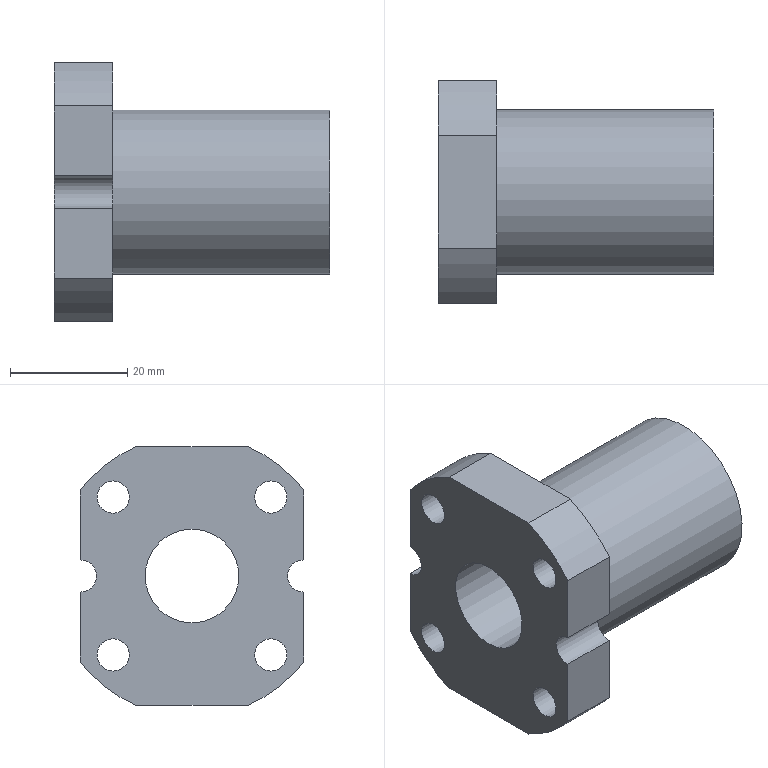Part | NX | 1 solid | 21 faces | box 47 x 38 x 44 mm | volume 27725 mm3 | cylinder 12 | plane 9 | commonest cylinder face diameters 5.5 x6 48 x4 16 x1 28 x1
STEP:
#1=CARTESIAN_POINT('',(0.,19.,14.663));
#2=VERTEX_POINT('',#1);
#3=CARTESIAN_POINT('',(0.,19.,2.75));
#4=VERTEX_POINT('',#3);
#5=CARTESIAN_POINT('',(0.,19.,14.663));
#6=DIRECTION('',(0.,0.,-1.));
#7=VECTOR('',#6,1.);
#8=LINE('',#5,#7);
#9=EDGE_CURVE('',#2,#4,#8,.T.);
#10=ORIENTED_EDGE('',*,*,#9,.F.);
#11=CARTESIAN_POINT('',(10.,19.,14.663));
#12=VERTEX_POINT('',#11);
#13=CARTESIAN_POINT('',(10.,19.,14.663));
#14=DIRECTION('',(-1.,0.,0.));
#15=VECTOR('',#14,1.);
#16=LINE('',#13,#15);
#17=EDGE_CURVE('',#12,#2,#16,.T.);
#18=ORIENTED_EDGE('',*,*,#17,.F.);
#19=CARTESIAN_POINT('',(10.,19.,2.75));
#20=VERTEX_POINT('',#19);
#21=CARTESIAN_POINT('',(10.,19.,14.663));
#22=DIRECTION('',(0.,0.,-1.));
#23=VECTOR('',#22,1.);
#24=LINE('',#21,#23);
#25=EDGE_CURVE('',#12,#20,#24,.T.);
#26=ORIENTED_EDGE('',*,*,#25,.T.);
#27=CARTESIAN_POINT('',(10.,19.,2.75));
#28=DIRECTION('',(-1.,0.,0.));
#29=VECTOR('',#28,1.);
#30=LINE('',#27,#29);
#31=EDGE_CURVE('',#20,#4,#30,.T.);
#32=ORIENTED_EDGE('',*,*,#31,.T.);
#33=EDGE_LOOP('',(#10,#18,#26,#32));
#34=FACE_OUTER_BOUND('',#33,.T.);
#35=CARTESIAN_POINT('',(10.,19.,14.663));
#36=DIRECTION('',(0.,1.,0.));
#37=DIRECTION('',(0.,0.,-1.));
#38=AXIS2_PLACEMENT_3D('',#35,#36,#37);
#39=PLANE('',#38);
#40=ADVANCED_FACE('',(#34),#39,.T.);
#41=CARTESIAN_POINT('',(0.,19.,-2.75));
#42=VERTEX_POINT('',#41);
#43=CARTESIAN_POINT('',(0.,19.,0.));
#44=DIRECTION('',(1.,0.,0.));
#45=DIRECTION('',(0.,0.,-1.));
#46=AXIS2_PLACEMENT_3D('',#43,#44,#45);
#47=CIRCLE('',#46,2.75);
#48=EDGE_CURVE('',#4,#42,#47,.T.);
#49=ORIENTED_EDGE('',*,*,#48,.F.);
#50=ORIENTED_EDGE('',*,*,#31,.F.);
#51=CARTESIAN_POINT('',(10.,19.,-2.75));
#52=VERTEX_POINT('',#51);
#53=CARTESIAN_POINT('',(10.,19.,0.));
#54=DIRECTION('',(1.,0.,0.));
#55=DIRECTION('',(0.,0.,-1.));
#56=AXIS2_PLACEMENT_3D('',#53,#54,#55);
#57=CIRCLE('',#56,2.75);
#58=EDGE_CURVE('',#20,#52,#57,.T.);
#59=ORIENTED_EDGE('',*,*,#58,.T.);
#60=CARTESIAN_POINT('',(10.,19.,-2.75));
#61=DIRECTION('',(-1.,0.,0.));
#62=VECTOR('',#61,1.);
#63=LINE('',#60,#62);
#64=EDGE_CURVE('',#52,#42,#63,.T.);
#65=ORIENTED_EDGE('',*,*,#64,.T.);
#66=EDGE_LOOP('',(#49,#50,#59,#65));
#67=FACE_OUTER_BOUND('',#66,.T.);
#68=CARTESIAN_POINT('',(10.,19.,0.));
#69=DIRECTION('',(-1.,0.,0.));
#70=DIRECTION('',(0.,0.,-1.));
#71=AXIS2_PLACEMENT_3D('',#68,#69,#70);
#72=CYLINDRICAL_SURFACE('',#71,2.75);
#73=ADVANCED_FACE('',(#67),#72,.F.);
#74=CARTESIAN_POINT('',(0.,19.,-14.663));
#75=VERTEX_POINT('',#74);
#76=CARTESIAN_POINT('',(0.,19.,-2.75));
#77=DIRECTION('',(0.,0.,-1.));
#78=VECTOR('',#77,1.);
#79=LINE('',#76,#78);
#80=EDGE_CURVE('',#42,#75,#79,.T.);
#81=ORIENTED_EDGE('',*,*,#80,.F.);
#82=ORIENTED_EDGE('',*,*,#64,.F.);
#83=CARTESIAN_POINT('',(10.,19.,-14.663));
#84=VERTEX_POINT('',#83);
#85=CARTESIAN_POINT('',(10.,19.,-2.75));
#86=DIRECTION('',(0.,0.,-1.));
#87=VECTOR('',#86,1.);
#88=LINE('',#85,#87);
#89=EDGE_CURVE('',#52,#84,#88,.T.);
#90=ORIENTED_EDGE('',*,*,#89,.T.);
#91=CARTESIAN_POINT('',(10.,19.,-14.663));
#92=DIRECTION('',(-1.,0.,0.));
#93=VECTOR('',#92,1.);
#94=LINE('',#91,#93);
#95=EDGE_CURVE('',#84,#75,#94,.T.);
#96=ORIENTED_EDGE('',*,*,#95,.T.);
#97=EDGE_LOOP('',(#81,#82,#90,#96));
#98=FACE_OUTER_BOUND('',#97,.T.);
#99=CARTESIAN_POINT('',(10.,19.,-2.75));
#100=DIRECTION('',(0.,1.,0.));
#101=DIRECTION('',(0.,0.,-1.));
#102=AXIS2_PLACEMENT_3D('',#99,#100,#101);
#103=PLANE('',#102);
#104=ADVANCED_FACE('',(#98),#103,.T.);
#105=CARTESIAN_POINT('',(0.,9.592,-22.));
#106=VERTEX_POINT('',#105);
#107=CARTESIAN_POINT('',(0.,0.,0.));
#108=DIRECTION('',(-1.,0.,0.));
#109=DIRECTION('',(0.,0.,-1.));
#110=AXIS2_PLACEMENT_3D('',#107,#108,#109);
#111=CIRCLE('',#110,24.);
#112=EDGE_CURVE('',#75,#106,#111,.T.);
#113=ORIENTED_EDGE('',*,*,#112,.F.);
#114=ORIENTED_EDGE('',*,*,#95,.F.);
#115=CARTESIAN_POINT('',(10.,9.592,-22.));
#116=VERTEX_POINT('',#115);
#117=CARTESIAN_POINT('',(10.,0.,0.));
#118=DIRECTION('',(-1.,0.,0.));
#119=DIRECTION('',(0.,0.,-1.));
#120=AXIS2_PLACEMENT_3D('',#117,#118,#119);
#121=CIRCLE('',#120,24.);
#122=EDGE_CURVE('',#84,#116,#121,.T.);
#123=ORIENTED_EDGE('',*,*,#122,.T.);
#124=CARTESIAN_POINT('',(10.,9.592,-22.));
#125=DIRECTION('',(-1.,0.,0.));
#126=VECTOR('',#125,1.);
#127=LINE('',#124,#126);
#128=EDGE_CURVE('',#116,#106,#127,.T.);
#129=ORIENTED_EDGE('',*,*,#128,.T.);
#130=EDGE_LOOP('',(#113,#114,#123,#129));
#131=FACE_OUTER_BOUND('',#130,.T.);
#132=CARTESIAN_POINT('',(10.,0.,0.));
#133=DIRECTION('',(-1.,0.,0.));
#134=DIRECTION('',(0.,0.,-1.));
#135=AXIS2_PLACEMENT_3D('',#132,#133,#134);
#136=CYLINDRICAL_SURFACE('',#135,24.);
#137=ADVANCED_FACE('',(#131),#136,.T.);
#138=CARTESIAN_POINT('',(0.,-9.592,-22.));
#139=VERTEX_POINT('',#138);
#140=CARTESIAN_POINT('',(0.,9.592,-22.));
#141=DIRECTION('',(0.,-1.,0.));
#142=VECTOR('',#141,1.);
#143=LINE('',#140,#142);
#144=EDGE_CURVE('',#106,#139,#143,.T.);
#145=ORIENTED_EDGE('',*,*,#144,.F.);
#146=ORIENTED_EDGE('',*,*,#128,.F.);
#147=CARTESIAN_POINT('',(10.,-9.592,-22.));
#148=VERTEX_POINT('',#147);
#149=CARTESIAN_POINT('',(10.,9.592,-22.));
#150=DIRECTION('',(0.,-1.,0.));
#151=VECTOR('',#150,1.);
#152=LINE('',#149,#151);
#153=EDGE_CURVE('',#116,#148,#152,.T.);
#154=ORIENTED_EDGE('',*,*,#153,.T.);
#155=CARTESIAN_POINT('',(10.,-9.592,-22.));
#156=DIRECTION('',(-1.,0.,0.));
#157=VECTOR('',#156,1.);
#158=LINE('',#155,#157);
#159=EDGE_CURVE('',#148,#139,#158,.T.);
#160=ORIENTED_EDGE('',*,*,#159,.T.);
#161=EDGE_LOOP('',(#145,#146,#154,#160));
#162=FACE_OUTER_BOUND('',#161,.T.);
#163=CARTESIAN_POINT('',(10.,9.592,-22.));
#164=DIRECTION('',(0.,0.,-1.));
#165=DIRECTION('',(0.,-1.,0.));
#166=AXIS2_PLACEMENT_3D('',#163,#164,#165);
#167=PLANE('',#166);
#168=ADVANCED_FACE('',(#162),#167,.T.);
#169=CARTESIAN_POINT('',(0.,-19.,-14.663));
#170=VERTEX_POINT('',#169);
#171=CARTESIAN_POINT('',(0.,0.,0.));
#172=DIRECTION('',(-1.,0.,0.));
#173=DIRECTION('',(0.,0.,-1.));
#174=AXIS2_PLACEMENT_3D('',#171,#172,#173);
#175=CIRCLE('',#174,24.);
#176=EDGE_CURVE('',#139,#170,#175,.T.);
#177=ORIENTED_EDGE('',*,*,#176,.F.);
#178=ORIENTED_EDGE('',*,*,#159,.F.);
#179=CARTESIAN_POINT('',(10.,-19.,-14.663));
#180=VERTEX_POINT('',#179);
#181=CARTESIAN_POINT('',(10.,0.,0.));
#182=DIRECTION('',(-1.,0.,0.));
#183=DIRECTION('',(0.,0.,-1.));
#184=AXIS2_PLACEMENT_3D('',#181,#182,#183);
#185=CIRCLE('',#184,24.);
#186=EDGE_CURVE('',#148,#180,#185,.T.);
#187=ORIENTED_EDGE('',*,*,#186,.T.);
#188=CARTESIAN_POINT('',(10.,-19.,-14.663));
#189=DIRECTION('',(-1.,0.,0.));
#190=VECTOR('',#189,1.);
#191=LINE('',#188,#190);
#192=EDGE_CURVE('',#180,#170,#191,.T.);
#193=ORIENTED_EDGE('',*,*,#192,.T.);
#194=EDGE_LOOP('',(#177,#178,#187,#193));
#195=FACE_OUTER_BOUND('',#194,.T.);
#196=CARTESIAN_POINT('',(10.,0.,0.));
#197=DIRECTION('',(-1.,0.,0.));
#198=DIRECTION('',(0.,0.,-1.));
#199=AXIS2_PLACEMENT_3D('',#196,#197,#198);
#200=CYLINDRICAL_SURFACE('',#199,24.);
#201=ADVANCED_FACE('',(#195),#200,.T.);
#202=CARTESIAN_POINT('',(0.,-19.,-2.75));
#203=VERTEX_POINT('',#202);
#204=CARTESIAN_POINT('',(0.,-19.,-14.663));
#205=DIRECTION('',(0.,0.,1.));
#206=VECTOR('',#205,1.);
#207=LINE('',#204,#206);
#208=EDGE_CURVE('',#170,#203,#207,.T.);
#209=ORIENTED_EDGE('',*,*,#208,.F.);
#210=ORIENTED_EDGE('',*,*,#192,.F.);
#211=CARTESIAN_POINT('',(10.,-19.,-2.75));
#212=VERTEX_POINT('',#211);
#213=CARTESIAN_POINT('',(10.,-19.,-14.663));
#214=DIRECTION('',(0.,0.,1.));
#215=VECTOR('',#214,1.);
#216=LINE('',#213,#215);
#217=EDGE_CURVE('',#180,#212,#216,.T.);
#218=ORIENTED_EDGE('',*,*,#217,.T.);
#219=CARTESIAN_POINT('',(10.,-19.,-2.75));
#220=DIRECTION('',(-1.,0.,0.));
#221=VECTOR('',#220,1.);
#222=LINE('',#219,#221);
#223=EDGE_CURVE('',#212,#203,#222,.T.);
#224=ORIENTED_EDGE('',*,*,#223,.T.);
#225=EDGE_LOOP('',(#209,#210,#218,#224));
#226=FACE_OUTER_BOUND('',#225,.T.);
#227=CARTESIAN_POINT('',(10.,-19.,-14.663));
#228=DIRECTION('',(0.,-1.,0.));
#229=DIRECTION('',(0.,0.,1.));
#230=AXIS2_PLACEMENT_3D('',#227,#228,#229);
#231=PLANE('',#230);
#232=ADVANCED_FACE('',(#226),#231,.T.);
#233=CARTESIAN_POINT('',(0.,-19.,2.75));
#234=VERTEX_POINT('',#233);
#235=CARTESIAN_POINT('',(0.,-19.,0.));
#236=DIRECTION('',(1.,0.,0.));
#237=DIRECTION('',(0.,0.,-1.));
#238=AXIS2_PLACEMENT_3D('',#235,#236,#237);
#239=CIRCLE('',#238,2.75);
#240=EDGE_CURVE('',#203,#234,#239,.T.);
#241=ORIENTED_EDGE('',*,*,#240,.F.);
#242=ORIENTED_EDGE('',*,*,#223,.F.);
#243=CARTESIAN_POINT('',(10.,-19.,2.75));
#244=VERTEX_POINT('',#243);
#245=CARTESIAN_POINT('',(10.,-19.,0.));
#246=DIRECTION('',(1.,0.,0.));
#247=DIRECTION('',(0.,0.,-1.));
#248=AXIS2_PLACEMENT_3D('',#245,#246,#247);
#249=CIRCLE('',#248,2.75);
#250=EDGE_CURVE('',#212,#244,#249,.T.);
#251=ORIENTED_EDGE('',*,*,#250,.T.);
#252=CARTESIAN_POINT('',(10.,-19.,2.75));
#253=DIRECTION('',(-1.,0.,0.));
#254=VECTOR('',#253,1.);
#255=LINE('',#252,#254);
#256=EDGE_CURVE('',#244,#234,#255,.T.);
#257=ORIENTED_EDGE('',*,*,#256,.T.);
#258=EDGE_LOOP('',(#241,#242,#251,#257));
#259=FACE_OUTER_BOUND('',#258,.T.);
#260=CARTESIAN_POINT('',(10.,-19.,0.));
#261=DIRECTION('',(-1.,0.,0.));
#262=DIRECTION('',(0.,0.,-1.));
#263=AXIS2_PLACEMENT_3D('',#260,#261,#262);
#264=CYLINDRICAL_SURFACE('',#263,2.75);
#265=ADVANCED_FACE('',(#259),#264,.F.);
#266=CARTESIAN_POINT('',(0.,-19.,14.663));
#267=VERTEX_POINT('',#266);
#268=CARTESIAN_POINT('',(0.,-19.,2.75));
#269=DIRECTION('',(0.,0.,1.));
#270=VECTOR('',#269,1.);
#271=LINE('',#268,#270);
#272=EDGE_CURVE('',#234,#267,#271,.T.);
#273=ORIENTED_EDGE('',*,*,#272,.F.);
#274=ORIENTED_EDGE('',*,*,#256,.F.);
#275=CARTESIAN_POINT('',(10.,-19.,14.663));
#276=VERTEX_POINT('',#275);
#277=CARTESIAN_POINT('',(10.,-19.,2.75));
#278=DIRECTION('',(0.,0.,1.));
#279=VECTOR('',#278,1.);
#280=LINE('',#277,#279);
#281=EDGE_CURVE('',#244,#276,#280,.T.);
#282=ORIENTED_EDGE('',*,*,#281,.T.);
#283=CARTESIAN_POINT('',(10.,-19.,14.663));
#284=DIRECTION('',(-1.,0.,0.));
#285=VECTOR('',#284,1.);
#286=LINE('',#283,#285);
#287=EDGE_CURVE('',#276,#267,#286,.T.);
#288=ORIENTED_EDGE('',*,*,#287,.T.);
#289=EDGE_LOOP('',(#273,#274,#282,#288));
#290=FACE_OUTER_BOUND('',#289,.T.);
#291=CARTESIAN_POINT('',(10.,-19.,2.75));
#292=DIRECTION('',(0.,-1.,0.));
#293=DIRECTION('',(0.,0.,1.));
#294=AXIS2_PLACEMENT_3D('',#291,#292,#293);
#295=PLANE('',#294);
#296=ADVANCED_FACE('',(#290),#295,.T.);
#297=CARTESIAN_POINT('',(0.,-9.592,22.));
#298=VERTEX_POINT('',#297);
#299=CARTESIAN_POINT('',(0.,0.,0.));
#300=DIRECTION('',(-1.,0.,0.));
#301=DIRECTION('',(0.,0.,-1.));
#302=AXIS2_PLACEMENT_3D('',#299,#300,#301);
#303=CIRCLE('',#302,24.);
#304=EDGE_CURVE('',#267,#298,#303,.T.);
#305=ORIENTED_EDGE('',*,*,#304,.F.);
#306=ORIENTED_EDGE('',*,*,#287,.F.);
#307=CARTESIAN_POINT('',(10.,-9.592,22.));
#308=VERTEX_POINT('',#307);
#309=CARTESIAN_POINT('',(10.,0.,0.));
#310=DIRECTION('',(-1.,0.,0.));
#311=DIRECTION('',(0.,0.,-1.));
#312=AXIS2_PLACEMENT_3D('',#309,#310,#311);
#313=CIRCLE('',#312,24.);
#314=EDGE_CURVE('',#276,#308,#313,.T.);
#315=ORIENTED_EDGE('',*,*,#314,.T.);
#316=CARTESIAN_POINT('',(10.,-9.592,22.));
#317=DIRECTION('',(-1.,0.,0.));
#318=VECTOR('',#317,1.);
#319=LINE('',#316,#318);
#320=EDGE_CURVE('',#308,#298,#319,.T.);
#321=ORIENTED_EDGE('',*,*,#320,.T.);
#322=EDGE_LOOP('',(#305,#306,#315,#321));
#323=FACE_OUTER_BOUND('',#322,.T.);
#324=CARTESIAN_POINT('',(10.,0.,0.));
#325=DIRECTION('',(-1.,0.,0.));
#326=DIRECTION('',(0.,0.,-1.));
#327=AXIS2_PLACEMENT_3D('',#324,#325,#326);
#328=CYLINDRICAL_SURFACE('',#327,24.);
#329=ADVANCED_FACE('',(#323),#328,.T.);
#330=CARTESIAN_POINT('',(0.,9.592,22.));
#331=VERTEX_POINT('',#330);
#332=CARTESIAN_POINT('',(0.,-9.592,22.));
#333=DIRECTION('',(0.,1.,0.));
#334=VECTOR('',#333,1.);
#335=LINE('',#332,#334);
#336=EDGE_CURVE('',#298,#331,#335,.T.);
#337=ORIENTED_EDGE('',*,*,#336,.F.);
#338=ORIENTED_EDGE('',*,*,#320,.F.);
#339=CARTESIAN_POINT('',(10.,9.592,22.));
#340=VERTEX_POINT('',#339);
#341=CARTESIAN_POINT('',(10.,-9.592,22.));
#342=DIRECTION('',(0.,1.,0.));
#343=VECTOR('',#342,1.);
#344=LINE('',#341,#343);
#345=EDGE_CURVE('',#308,#340,#344,.T.);
#346=ORIENTED_EDGE('',*,*,#345,.T.);
#347=CARTESIAN_POINT('',(10.,9.592,22.));
#348=DIRECTION('',(-1.,0.,0.));
#349=VECTOR('',#348,1.);
#350=LINE('',#347,#349);
#351=EDGE_CURVE('',#340,#331,#350,.T.);
#352=ORIENTED_EDGE('',*,*,#351,.T.);
#353=EDGE_LOOP('',(#337,#338,#346,#352));
#354=FACE_OUTER_BOUND('',#353,.T.);
#355=CARTESIAN_POINT('',(10.,-9.592,22.));
#356=DIRECTION('',(0.,0.,1.));
#357=DIRECTION('',(0.,1.,0.));
#358=AXIS2_PLACEMENT_3D('',#355,#356,#357);
#359=PLANE('',#358);
#360=ADVANCED_FACE('',(#354),#359,.T.);
#361=CARTESIAN_POINT('',(0.,13.435,-16.185));
#362=VERTEX_POINT('',#361);
#363=CARTESIAN_POINT('',(0.,13.435,-13.435));
#364=DIRECTION('',(-1.,0.,0.));
#365=DIRECTION('',(0.,0.,-1.));
#366=AXIS2_PLACEMENT_3D('',#363,#364,#365);
#367=CIRCLE('',#366,2.75);
#368=EDGE_CURVE('',#362,#362,#367,.T.);
#369=ORIENTED_EDGE('',*,*,#368,.T.);
#370=EDGE_LOOP('',(#369));
#371=FACE_BOUND('',#370,.T.);
#372=CARTESIAN_POINT('',(10.,13.435,-16.185));
#373=VERTEX_POINT('',#372);
#374=CARTESIAN_POINT('',(10.,13.435,-13.435));
#375=DIRECTION('',(-1.,0.,0.));
#376=DIRECTION('',(0.,0.,-1.));
#377=AXIS2_PLACEMENT_3D('',#374,#375,#376);
#378=CIRCLE('',#377,2.75);
#379=EDGE_CURVE('',#373,#373,#378,.T.);
#380=ORIENTED_EDGE('',*,*,#379,.F.);
#381=EDGE_LOOP('',(#380));
#382=FACE_BOUND('',#381,.T.);
#383=CARTESIAN_POINT('',(10.,13.435,-13.435));
#384=DIRECTION('',(-1.,0.,0.));
#385=DIRECTION('',(0.,0.,-1.));
#386=AXIS2_PLACEMENT_3D('',#383,#384,#385);
#387=CYLINDRICAL_SURFACE('',#386,2.75);
#388=ADVANCED_FACE('',(#371,#382),#387,.F.);
#389=CARTESIAN_POINT('',(0.,-13.435,10.685));
#390=VERTEX_POINT('',#389);
#391=CARTESIAN_POINT('',(0.,-13.435,13.435));
#392=DIRECTION('',(-1.,0.,0.));
#393=DIRECTION('',(0.,0.,-1.));
#394=AXIS2_PLACEMENT_3D('',#391,#392,#393);
#395=CIRCLE('',#394,2.75);
#396=EDGE_CURVE('',#390,#390,#395,.T.);
#397=ORIENTED_EDGE('',*,*,#396,.T.);
#398=EDGE_LOOP('',(#397));
#399=FACE_BOUND('',#398,.T.);
#400=CARTESIAN_POINT('',(10.,-13.435,10.685));
#401=VERTEX_POINT('',#400);
#402=CARTESIAN_POINT('',(10.,-13.435,13.435));
#403=DIRECTION('',(-1.,0.,0.));
#404=DIRECTION('',(0.,0.,-1.));
#405=AXIS2_PLACEMENT_3D('',#402,#403,#404);
#406=CIRCLE('',#405,2.75);
#407=EDGE_CURVE('',#401,#401,#406,.T.);
#408=ORIENTED_EDGE('',*,*,#407,.F.);
#409=EDGE_LOOP('',(#408));
#410=FACE_BOUND('',#409,.T.);
#411=CARTESIAN_POINT('',(10.,-13.435,13.435));
#412=DIRECTION('',(-1.,0.,0.));
#413=DIRECTION('',(0.,0.,-1.));
#414=AXIS2_PLACEMENT_3D('',#411,#412,#413);
#415=CYLINDRICAL_SURFACE('',#414,2.75);
#416=ADVANCED_FACE('',(#399,#410),#415,.F.);
#417=CARTESIAN_POINT('',(0.,-13.435,-16.185));
#418=VERTEX_POINT('',#417);
#419=CARTESIAN_POINT('',(0.,-13.435,-13.435));
#420=DIRECTION('',(-1.,0.,0.));
#421=DIRECTION('',(0.,0.,-1.));
#422=AXIS2_PLACEMENT_3D('',#419,#420,#421);
#423=CIRCLE('',#422,2.75);
#424=EDGE_CURVE('',#418,#418,#423,.T.);
#425=ORIENTED_EDGE('',*,*,#424,.T.);
#426=EDGE_LOOP('',(#425));
#427=FACE_BOUND('',#426,.T.);
#428=CARTESIAN_POINT('',(10.,-13.435,-16.185));
#429=VERTEX_POINT('',#428);
#430=CARTESIAN_POINT('',(10.,-13.435,-13.435));
#431=DIRECTION('',(-1.,0.,0.));
#432=DIRECTION('',(0.,0.,-1.));
#433=AXIS2_PLACEMENT_3D('',#430,#431,#432);
#434=CIRCLE('',#433,2.75);
#435=EDGE_CURVE('',#429,#429,#434,.T.);
#436=ORIENTED_EDGE('',*,*,#435,.F.);
#437=EDGE_LOOP('',(#436));
#438=FACE_BOUND('',#437,.T.);
#439=CARTESIAN_POINT('',(10.,-13.435,-13.435));
#440=DIRECTION('',(-1.,0.,0.));
#441=DIRECTION('',(0.,0.,-1.));
#442=AXIS2_PLACEMENT_3D('',#439,#440,#441);
#443=CYLINDRICAL_SURFACE('',#442,2.75);
#444=ADVANCED_FACE('',(#427,#438),#443,.F.);
#445=CARTESIAN_POINT('',(0.,0.,0.));
#446=DIRECTION('',(-1.,0.,0.));
#447=DIRECTION('',(0.,0.,-1.));
#448=AXIS2_PLACEMENT_3D('',#445,#446,#447);
#449=CIRCLE('',#448,24.);
#450=EDGE_CURVE('',#331,#2,#449,.T.);
#451=ORIENTED_EDGE('',*,*,#450,.F.);
#452=ORIENTED_EDGE('',*,*,#351,.F.);
#453=CARTESIAN_POINT('',(10.,0.,0.));
#454=DIRECTION('',(-1.,0.,0.));
#455=DIRECTION('',(0.,0.,-1.));
#456=AXIS2_PLACEMENT_3D('',#453,#454,#455);
#457=CIRCLE('',#456,24.);
#458=EDGE_CURVE('',#340,#12,#457,.T.);
#459=ORIENTED_EDGE('',*,*,#458,.T.);
#460=ORIENTED_EDGE('',*,*,#17,.T.);
#461=EDGE_LOOP('',(#451,#452,#459,#460));
#462=FACE_OUTER_BOUND('',#461,.T.);
#463=CARTESIAN_POINT('',(10.,0.,0.));
#464=DIRECTION('',(-1.,0.,0.));
#465=DIRECTION('',(0.,0.,-1.));
#466=AXIS2_PLACEMENT_3D('',#463,#464,#465);
#467=CYLINDRICAL_SURFACE('',#466,24.);
#468=ADVANCED_FACE('',(#462),#467,.T.);
#469=CARTESIAN_POINT('',(0.,13.435,10.685));
#470=VERTEX_POINT('',#469);
#471=CARTESIAN_POINT('',(0.,13.435,13.435));
#472=DIRECTION('',(-1.,0.,0.));
#473=DIRECTION('',(0.,0.,-1.));
#474=AXIS2_PLACEMENT_3D('',#471,#472,#473);
#475=CIRCLE('',#474,2.75);
#476=EDGE_CURVE('',#470,#470,#475,.T.);
#477=ORIENTED_EDGE('',*,*,#476,.T.);
#478=EDGE_LOOP('',(#477));
#479=FACE_BOUND('',#478,.T.);
#480=CARTESIAN_POINT('',(10.,13.435,10.685));
#481=VERTEX_POINT('',#480);
#482=CARTESIAN_POINT('',(10.,13.435,13.435));
#483=DIRECTION('',(-1.,0.,0.));
#484=DIRECTION('',(0.,0.,-1.));
#485=AXIS2_PLACEMENT_3D('',#482,#483,#484);
#486=CIRCLE('',#485,2.75);
#487=EDGE_CURVE('',#481,#481,#486,.T.);
#488=ORIENTED_EDGE('',*,*,#487,.F.);
#489=EDGE_LOOP('',(#488));
#490=FACE_BOUND('',#489,.T.);
#491=CARTESIAN_POINT('',(10.,13.435,13.435));
#492=DIRECTION('',(-1.,0.,0.));
#493=DIRECTION('',(0.,0.,-1.));
#494=AXIS2_PLACEMENT_3D('',#491,#492,#493);
#495=CYLINDRICAL_SURFACE('',#494,2.75);
#496=ADVANCED_FACE('',(#479,#490),#495,.F.);
#497=CARTESIAN_POINT('',(10.,0.,-14.));
#498=VERTEX_POINT('',#497);
#499=CARTESIAN_POINT('',(10.,0.,0.));
#500=DIRECTION('',(-1.,0.,0.));
#501=DIRECTION('',(0.,0.,-1.));
#502=AXIS2_PLACEMENT_3D('',#499,#500,#501);
#503=CIRCLE('',#502,14.);
#504=EDGE_CURVE('',#498,#498,#503,.T.);
#505=ORIENTED_EDGE('',*,*,#504,.T.);
#506=EDGE_LOOP('',(#505));
#507=FACE_BOUND('',#506,.T.);
#508=ORIENTED_EDGE('',*,*,#25,.F.);
#509=ORIENTED_EDGE('',*,*,#458,.F.);
#510=ORIENTED_EDGE('',*,*,#345,.F.);
#511=ORIENTED_EDGE('',*,*,#314,.F.);
#512=ORIENTED_EDGE('',*,*,#281,.F.);
#513=ORIENTED_EDGE('',*,*,#250,.F.);
#514=ORIENTED_EDGE('',*,*,#217,.F.);
#515=ORIENTED_EDGE('',*,*,#186,.F.);
#516=ORIENTED_EDGE('',*,*,#153,.F.);
#517=ORIENTED_EDGE('',*,*,#122,.F.);
#518=ORIENTED_EDGE('',*,*,#89,.F.);
#519=ORIENTED_EDGE('',*,*,#58,.F.);
#520=EDGE_LOOP('',(#508,#509,#510,#511,#512,#513,#514,#515,#516,#517,#518,#519));
#521=FACE_BOUND('',#520,.T.);
#522=ORIENTED_EDGE('',*,*,#435,.T.);
#523=EDGE_LOOP('',(#522));
#524=FACE_BOUND('',#523,.T.);
#525=ORIENTED_EDGE('',*,*,#407,.T.);
#526=EDGE_LOOP('',(#525));
#527=FACE_BOUND('',#526,.T.);
#528=ORIENTED_EDGE('',*,*,#379,.T.);
#529=EDGE_LOOP('',(#528));
#530=FACE_BOUND('',#529,.T.);
#531=ORIENTED_EDGE('',*,*,#487,.T.);
#532=EDGE_LOOP('',(#531));
#533=FACE_BOUND('',#532,.T.);
#534=CARTESIAN_POINT('',(10.,19.,0.));
#535=DIRECTION('',(1.,0.,0.));
#536=DIRECTION('',(0.,0.,1.));
#537=AXIS2_PLACEMENT_3D('',#534,#535,#536);
#538=PLANE('',#537);
#539=ADVANCED_FACE('',(#507,#521,#524,#527,#530,#533),#538,.T.);
#540=CARTESIAN_POINT('',(0.,0.,8.));
#541=VERTEX_POINT('',#540);
#542=CARTESIAN_POINT('',(0.,0.,0.));
#543=DIRECTION('',(1.,0.,0.));
#544=DIRECTION('',(0.,0.,1.));
#545=AXIS2_PLACEMENT_3D('',#542,#543,#544);
#546=CIRCLE('',#545,8.);
#547=EDGE_CURVE('',#541,#541,#546,.T.);
#548=ORIENTED_EDGE('',*,*,#547,.T.);
#549=EDGE_LOOP('',(#548));
#550=FACE_BOUND('',#549,.T.);
#551=ORIENTED_EDGE('',*,*,#9,.T.);
#552=ORIENTED_EDGE('',*,*,#48,.T.);
#553=ORIENTED_EDGE('',*,*,#80,.T.);
#554=ORIENTED_EDGE('',*,*,#112,.T.);
#555=ORIENTED_EDGE('',*,*,#144,.T.);
#556=ORIENTED_EDGE('',*,*,#176,.T.);
#557=ORIENTED_EDGE('',*,*,#208,.T.);
#558=ORIENTED_EDGE('',*,*,#240,.T.);
#559=ORIENTED_EDGE('',*,*,#272,.T.);
#560=ORIENTED_EDGE('',*,*,#304,.T.);
#561=ORIENTED_EDGE('',*,*,#336,.T.);
#562=ORIENTED_EDGE('',*,*,#450,.T.);
#563=EDGE_LOOP('',(#551,#552,#553,#554,#555,#556,#557,#558,#559,#560,#561,#562));
#564=FACE_BOUND('',#563,.T.);
#565=ORIENTED_EDGE('',*,*,#424,.F.);
#566=EDGE_LOOP('',(#565));
#567=FACE_BOUND('',#566,.T.);
#568=ORIENTED_EDGE('',*,*,#396,.F.);
#569=EDGE_LOOP('',(#568));
#570=FACE_BOUND('',#569,.T.);
#571=ORIENTED_EDGE('',*,*,#368,.F.);
#572=EDGE_LOOP('',(#571));
#573=FACE_BOUND('',#572,.T.);
#574=ORIENTED_EDGE('',*,*,#476,.F.);
#575=EDGE_LOOP('',(#574));
#576=FACE_BOUND('',#575,.T.);
#577=CARTESIAN_POINT('',(0.,19.,0.));
#578=DIRECTION('',(1.,0.,0.));
#579=DIRECTION('',(0.,0.,1.));
#580=AXIS2_PLACEMENT_3D('',#577,#578,#579);
#581=PLANE('',#580);
#582=ADVANCED_FACE('',(#550,#564,#567,#570,#573,#576),#581,.F.);
#583=ORIENTED_EDGE('',*,*,#504,.F.);
#584=EDGE_LOOP('',(#583));
#585=FACE_BOUND('',#584,.T.);
#586=CARTESIAN_POINT('',(47.,0.,-14.));
#587=VERTEX_POINT('',#586);
#588=CARTESIAN_POINT('',(47.,0.,0.));
#589=DIRECTION('',(1.,0.,0.));
#590=DIRECTION('',(0.,0.,-1.));
#591=AXIS2_PLACEMENT_3D('',#588,#589,#590);
#592=CIRCLE('',#591,14.);
#593=EDGE_CURVE('',#587,#587,#592,.T.);
#594=ORIENTED_EDGE('',*,*,#593,.F.);
#595=EDGE_LOOP('',(#594));
#596=FACE_BOUND('',#595,.T.);
#597=CARTESIAN_POINT('',(47.,0.,0.));
#598=DIRECTION('',(-1.,0.,0.));
#599=DIRECTION('',(0.,0.,-1.));
#600=AXIS2_PLACEMENT_3D('',#597,#598,#599);
#601=CYLINDRICAL_SURFACE('',#600,14.);
#602=ADVANCED_FACE('',(#585,#596),#601,.T.);
#603=CARTESIAN_POINT('',(47.,0.,8.));
#604=VERTEX_POINT('',#603);
#605=CARTESIAN_POINT('',(47.,0.,0.));
#606=DIRECTION('',(1.,0.,0.));
#607=DIRECTION('',(0.,0.,1.));
#608=AXIS2_PLACEMENT_3D('',#605,#606,#607);
#609=CIRCLE('',#608,8.);
#610=EDGE_CURVE('',#604,#604,#609,.T.);
#611=ORIENTED_EDGE('',*,*,#610,.F.);
#612=EDGE_LOOP('',(#611));
#613=FACE_BOUND('',#612,.T.);
#614=ORIENTED_EDGE('',*,*,#593,.T.);
#615=EDGE_LOOP('',(#614));
#616=FACE_BOUND('',#615,.T.);
#617=CARTESIAN_POINT('',(47.,0.,0.));
#618=DIRECTION('',(1.,0.,0.));
#619=DIRECTION('',(0.,0.,1.));
#620=AXIS2_PLACEMENT_3D('',#617,#618,#619);
#621=PLANE('',#620);
#622=ADVANCED_FACE('',(#613,#616),#621,.T.);
#623=ORIENTED_EDGE('',*,*,#547,.F.);
#624=EDGE_LOOP('',(#623));
#625=FACE_BOUND('',#624,.T.);
#626=ORIENTED_EDGE('',*,*,#610,.T.);
#627=EDGE_LOOP('',(#626));
#628=FACE_BOUND('',#627,.T.);
#629=CARTESIAN_POINT('',(47.,0.,0.));
#630=DIRECTION('',(-1.,0.,0.));
#631=DIRECTION('',(0.,0.,-1.));
#632=AXIS2_PLACEMENT_3D('',#629,#630,#631);
#633=CYLINDRICAL_SURFACE('',#632,8.);
#634=ADVANCED_FACE('',(#625,#628),#633,.F.);
#635=CLOSED_SHELL('',(#40,#73,#104,#137,#168,#201,#232,#265,#296,#329,#360,#388,#416,#444,#468,#496,#539,#582,#602,#622,#634));
#636=MANIFOLD_SOLID_BREP('',#635);
#637=(LENGTH_UNIT()NAMED_UNIT(*)SI_UNIT(.MILLI.,.METRE.));
#638=UNCERTAINTY_MEASURE_WITH_UNIT(LENGTH_MEASURE(0.00002),#637,'','');
#639=(NAMED_UNIT(*)PLANE_ANGLE_UNIT()SI_UNIT($,.RADIAN.));
#640=PLANE_ANGLE_MEASURE_WITH_UNIT(PLANE_ANGLE_MEASURE(0.01745),#639);
#641=DIMENSIONAL_EXPONENTS(0.,0.,0.,0.,0.,0.,0.);
#642=(CONVERSION_BASED_UNIT('DEGREE',#640)NAMED_UNIT(#641)PLANE_ANGLE_UNIT());
#643=(NAMED_UNIT(*)SI_UNIT($,.STERADIAN.)SOLID_ANGLE_UNIT());
#644=(GEOMETRIC_REPRESENTATION_CONTEXT(3)GLOBAL_UNCERTAINTY_ASSIGNED_CONTEXT((#638))GLOBAL_UNIT_ASSIGNED_CONTEXT((#637,#642,#643))REPRESENTATION_CONTEXT('',''));
#645=ADVANCED_BREP_SHAPE_REPRESENTATION('',(#636),#644);